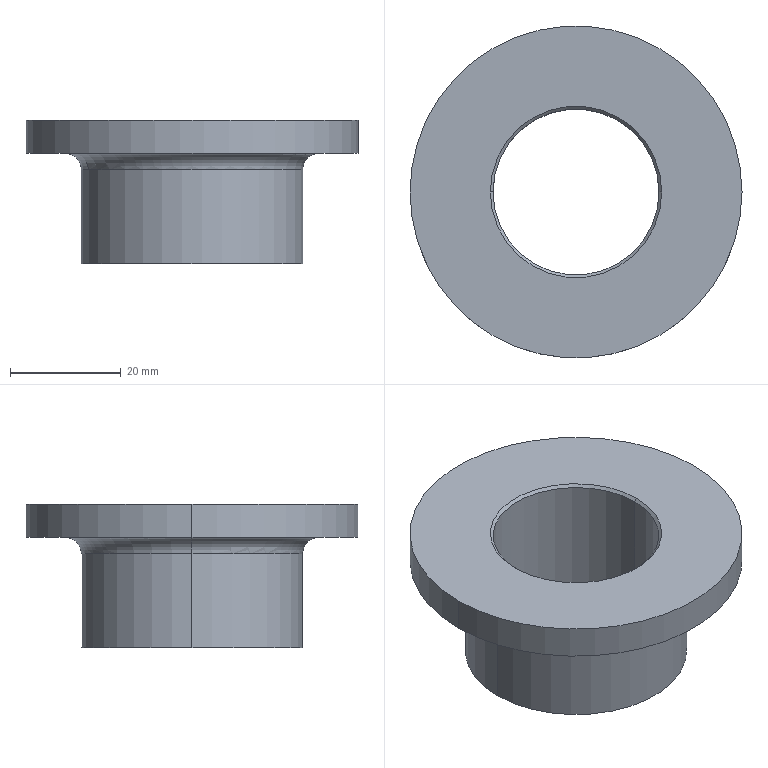Part | SolidWorks | features Chamfer 1, Extrusion 1, Fillet 1, ICE 1 | 1 solid | 15 faces | box 60 x 60 x 26 mm | volume 23946 mm3 | cylinder 6 | cone 4 | plane 3 | torus 2 | commonest cylinder face diameters 30 x2 40 x2 60 x2
STEP:
#1=CARTESIAN_POINT('',(15.,0.,0.5));
#2=VERTEX_POINT('',#1);
#3=CARTESIAN_POINT('',(-15.,0.,0.5));
#4=VERTEX_POINT('',#3);
#5=CARTESIAN_POINT('',(0.,0.,0.5));
#6=DIRECTION('',(0.,0.,-1.));
#7=DIRECTION('',(1.,0.,0.));
#8=AXIS2_PLACEMENT_3D('',#5,#6,#7);
#9=CIRCLE('',#8,15.);
#10=EDGE_CURVE('',#2,#4,#9,.T.);
#11=ORIENTED_EDGE('',*,*,#10,.F.);
#12=CARTESIAN_POINT('',(15.5,0.,0.));
#13=VERTEX_POINT('',#12);
#14=CARTESIAN_POINT('',(15.5,0.,0.));
#15=DIRECTION('',(0.7071,0.,-0.7071));
#16=VECTOR('',#15,1000.);
#17=LINE('',#14,#16);
#18=EDGE_CURVE('',#2,#13,#17,.T.);
#19=ORIENTED_EDGE('',*,*,#18,.T.);
#20=CARTESIAN_POINT('',(-15.5,0.,0.));
#21=VERTEX_POINT('',#20);
#22=CARTESIAN_POINT('',(0.,0.,0.));
#23=DIRECTION('',(0.,0.,1.));
#24=DIRECTION('',(1.,0.,0.));
#25=AXIS2_PLACEMENT_3D('',#22,#23,#24);
#26=CIRCLE('',#25,15.5);
#27=EDGE_CURVE('',#21,#13,#26,.T.);
#28=ORIENTED_EDGE('',*,*,#27,.F.);
#29=CARTESIAN_POINT('',(-15.5,0.,0.));
#30=DIRECTION('',(-0.7071,0.,-0.7071));
#31=VECTOR('',#30,1000.);
#32=LINE('',#29,#31);
#33=EDGE_CURVE('',#4,#21,#32,.T.);
#34=ORIENTED_EDGE('',*,*,#33,.F.);
#35=EDGE_LOOP('',(#11,#19,#28,#34));
#36=FACE_OUTER_BOUND('',#35,.T.);
#37=CARTESIAN_POINT('',(0.,0.,0.));
#38=DIRECTION('',(0.,0.,-1.));
#39=DIRECTION('',(-1.,0.,0.));
#40=AXIS2_PLACEMENT_3D('',#37,#38,#39);
#41=CONICAL_SURFACE('',#40,15.5,0.7854);
#42=ADVANCED_FACE('',(#36),#41,.F.);
#43=CARTESIAN_POINT('',(-15.,0.,25.5));
#44=VERTEX_POINT('',#43);
#45=CARTESIAN_POINT('',(15.,0.,25.5));
#46=VERTEX_POINT('',#45);
#47=CARTESIAN_POINT('',(0.,0.,25.5));
#48=DIRECTION('',(0.,0.,1.));
#49=DIRECTION('',(1.,0.,0.));
#50=AXIS2_PLACEMENT_3D('',#47,#48,#49);
#51=CIRCLE('',#50,15.);
#52=EDGE_CURVE('',#44,#46,#51,.T.);
#53=ORIENTED_EDGE('',*,*,#52,.F.);
#54=CARTESIAN_POINT('',(-15.5,0.,26.));
#55=VERTEX_POINT('',#54);
#56=CARTESIAN_POINT('',(-15.,0.,25.5));
#57=DIRECTION('',(-0.7071,0.,0.7071));
#58=VECTOR('',#57,1000.);
#59=LINE('',#56,#58);
#60=EDGE_CURVE('',#44,#55,#59,.T.);
#61=ORIENTED_EDGE('',*,*,#60,.T.);
#62=CARTESIAN_POINT('',(15.5,0.,26.));
#63=VERTEX_POINT('',#62);
#64=CARTESIAN_POINT('',(0.,0.,26.));
#65=DIRECTION('',(0.,0.,-1.));
#66=DIRECTION('',(1.,0.,0.));
#67=AXIS2_PLACEMENT_3D('',#64,#65,#66);
#68=CIRCLE('',#67,15.5);
#69=EDGE_CURVE('',#63,#55,#68,.T.);
#70=ORIENTED_EDGE('',*,*,#69,.F.);
#71=CARTESIAN_POINT('',(15.,0.,25.5));
#72=DIRECTION('',(0.7071,0.,0.7071));
#73=VECTOR('',#72,1000.);
#74=LINE('',#71,#73);
#75=EDGE_CURVE('',#46,#63,#74,.T.);
#76=ORIENTED_EDGE('',*,*,#75,.F.);
#77=EDGE_LOOP('',(#53,#61,#70,#76));
#78=FACE_OUTER_BOUND('',#77,.T.);
#79=CARTESIAN_POINT('',(0.,0.,25.5));
#80=DIRECTION('',(0.,0.,1.));
#81=DIRECTION('',(1.,0.,0.));
#82=AXIS2_PLACEMENT_3D('',#79,#80,#81);
#83=CONICAL_SURFACE('',#82,15.,0.7854);
#84=ADVANCED_FACE('',(#78),#83,.F.);
#85=CARTESIAN_POINT('',(-23.,0.,20.));
#86=VERTEX_POINT('',#85);
#87=CARTESIAN_POINT('',(23.,0.,20.));
#88=VERTEX_POINT('',#87);
#89=CARTESIAN_POINT('',(0.,0.,20.));
#90=DIRECTION('',(0.,0.,1.));
#91=DIRECTION('',(1.,0.,0.));
#92=AXIS2_PLACEMENT_3D('',#89,#90,#91);
#93=CIRCLE('',#92,23.);
#94=EDGE_CURVE('',#86,#88,#93,.T.);
#95=ORIENTED_EDGE('',*,*,#94,.F.);
#96=CARTESIAN_POINT('',(-20.,0.,17.));
#97=VERTEX_POINT('',#96);
#98=CARTESIAN_POINT('',(-23.,0.,17.));
#99=DIRECTION('',(0.,1.,0.));
#100=DIRECTION('',(-1.,0.,0.));
#101=AXIS2_PLACEMENT_3D('',#98,#99,#100);
#102=CIRCLE('',#101,3.);
#103=EDGE_CURVE('',#86,#97,#102,.T.);
#104=ORIENTED_EDGE('',*,*,#103,.T.);
#105=CARTESIAN_POINT('',(20.,0.,17.));
#106=VERTEX_POINT('',#105);
#107=CARTESIAN_POINT('',(0.,0.,17.));
#108=DIRECTION('',(0.,0.,-1.));
#109=DIRECTION('',(1.,0.,0.));
#110=AXIS2_PLACEMENT_3D('',#107,#108,#109);
#111=CIRCLE('',#110,20.);
#112=EDGE_CURVE('',#106,#97,#111,.T.);
#113=ORIENTED_EDGE('',*,*,#112,.F.);
#114=CARTESIAN_POINT('',(23.,0.,17.));
#115=DIRECTION('',(0.,-1.,0.));
#116=DIRECTION('',(0.,0.,-1.));
#117=AXIS2_PLACEMENT_3D('',#114,#115,#116);
#118=CIRCLE('',#117,3.);
#119=EDGE_CURVE('',#88,#106,#118,.T.);
#120=ORIENTED_EDGE('',*,*,#119,.F.);
#121=EDGE_LOOP('',(#95,#104,#113,#120));
#122=FACE_OUTER_BOUND('',#121,.T.);
#123=CARTESIAN_POINT('',(0.,0.,17.));
#124=DIRECTION('',(0.,0.,1.));
#125=DIRECTION('',(1.,0.,0.));
#126=AXIS2_PLACEMENT_3D('',#123,#124,#125);
#127=TOROIDAL_SURFACE('',#126,23.,3.);
#128=ADVANCED_FACE('',(#122),#127,.F.);
#129=CARTESIAN_POINT('',(30.,0.,20.));
#130=VERTEX_POINT('',#129);
#131=CARTESIAN_POINT('',(-30.,0.,20.));
#132=VERTEX_POINT('',#131);
#133=CARTESIAN_POINT('',(0.,0.,20.));
#134=DIRECTION('',(0.,0.,1.));
#135=DIRECTION('',(1.,0.,0.));
#136=AXIS2_PLACEMENT_3D('',#133,#134,#135);
#137=CIRCLE('',#136,30.);
#138=EDGE_CURVE('',#130,#132,#137,.T.);
#139=ORIENTED_EDGE('',*,*,#138,.T.);
#140=CARTESIAN_POINT('',(-30.,0.,26.));
#141=VERTEX_POINT('',#140);
#142=CARTESIAN_POINT('',(-30.,0.,20.));
#143=DIRECTION('',(0.,0.,1.));
#144=VECTOR('',#143,1000.);
#145=LINE('',#142,#144);
#146=EDGE_CURVE('',#132,#141,#145,.T.);
#147=ORIENTED_EDGE('',*,*,#146,.T.);
#148=CARTESIAN_POINT('',(30.,0.,26.));
#149=VERTEX_POINT('',#148);
#150=CARTESIAN_POINT('',(0.,0.,26.));
#151=DIRECTION('',(0.,0.,1.));
#152=DIRECTION('',(1.,0.,0.));
#153=AXIS2_PLACEMENT_3D('',#150,#151,#152);
#154=CIRCLE('',#153,30.);
#155=EDGE_CURVE('',#149,#141,#154,.T.);
#156=ORIENTED_EDGE('',*,*,#155,.F.);
#157=CARTESIAN_POINT('',(30.,0.,20.));
#158=DIRECTION('',(0.,0.,1.));
#159=VECTOR('',#158,1000.);
#160=LINE('',#157,#159);
#161=EDGE_CURVE('',#130,#149,#160,.T.);
#162=ORIENTED_EDGE('',*,*,#161,.F.);
#163=EDGE_LOOP('',(#139,#147,#156,#162));
#164=FACE_OUTER_BOUND('',#163,.T.);
#165=CARTESIAN_POINT('',(0.,0.,20.));
#166=DIRECTION('',(0.,0.,1.));
#167=DIRECTION('',(1.,0.,0.));
#168=AXIS2_PLACEMENT_3D('',#165,#166,#167);
#169=CYLINDRICAL_SURFACE('',#168,30.);
#170=ADVANCED_FACE('',(#164),#169,.T.);
#171=ORIENTED_EDGE('',*,*,#52,.T.);
#172=CARTESIAN_POINT('',(15.,0.,26.));
#173=DIRECTION('',(0.,0.,-1.));
#174=VECTOR('',#173,1000.);
#175=LINE('',#172,#174);
#176=EDGE_CURVE('',#46,#2,#175,.T.);
#177=ORIENTED_EDGE('',*,*,#176,.T.);
#178=ORIENTED_EDGE('',*,*,#10,.T.);
#179=CARTESIAN_POINT('',(-15.,0.,26.));
#180=DIRECTION('',(0.,0.,-1.));
#181=VECTOR('',#180,1000.);
#182=LINE('',#179,#181);
#183=EDGE_CURVE('',#44,#4,#182,.T.);
#184=ORIENTED_EDGE('',*,*,#183,.F.);
#185=EDGE_LOOP('',(#171,#177,#178,#184));
#186=FACE_OUTER_BOUND('',#185,.T.);
#187=CARTESIAN_POINT('',(0.,0.,26.));
#188=DIRECTION('',(0.,0.,-1.));
#189=DIRECTION('',(-1.,0.,0.));
#190=AXIS2_PLACEMENT_3D('',#187,#188,#189);
#191=CYLINDRICAL_SURFACE('',#190,15.);
#192=ADVANCED_FACE('',(#186),#191,.F.);
#193=CARTESIAN_POINT('',(0.,0.,17.));
#194=DIRECTION('',(0.,0.,-1.));
#195=DIRECTION('',(1.,0.,0.));
#196=AXIS2_PLACEMENT_3D('',#193,#194,#195);
#197=CIRCLE('',#196,20.);
#198=EDGE_CURVE('',#97,#106,#197,.T.);
#199=ORIENTED_EDGE('',*,*,#198,.T.);
#200=CARTESIAN_POINT('',(20.,0.,0.));
#201=VERTEX_POINT('',#200);
#202=CARTESIAN_POINT('',(20.,0.,26.));
#203=DIRECTION('',(0.,0.,-1.));
#204=VECTOR('',#203,1000.);
#205=LINE('',#202,#204);
#206=EDGE_CURVE('',#106,#201,#205,.T.);
#207=ORIENTED_EDGE('',*,*,#206,.T.);
#208=CARTESIAN_POINT('',(-20.,0.,0.));
#209=VERTEX_POINT('',#208);
#210=CARTESIAN_POINT('',(0.,0.,0.));
#211=DIRECTION('',(0.,0.,1.));
#212=DIRECTION('',(1.,0.,0.));
#213=AXIS2_PLACEMENT_3D('',#210,#211,#212);
#214=CIRCLE('',#213,20.);
#215=EDGE_CURVE('',#201,#209,#214,.T.);
#216=ORIENTED_EDGE('',*,*,#215,.T.);
#217=CARTESIAN_POINT('',(-20.,0.,26.));
#218=DIRECTION('',(0.,0.,-1.));
#219=VECTOR('',#218,1000.);
#220=LINE('',#217,#219);
#221=EDGE_CURVE('',#97,#209,#220,.T.);
#222=ORIENTED_EDGE('',*,*,#221,.F.);
#223=EDGE_LOOP('',(#199,#207,#216,#222));
#224=FACE_OUTER_BOUND('',#223,.T.);
#225=CARTESIAN_POINT('',(0.,0.,26.));
#226=DIRECTION('',(0.,0.,-1.));
#227=DIRECTION('',(-1.,0.,0.));
#228=AXIS2_PLACEMENT_3D('',#225,#226,#227);
#229=CYLINDRICAL_SURFACE('',#228,20.);
#230=ADVANCED_FACE('',(#224),#229,.T.);
#231=ORIENTED_EDGE('',*,*,#206,.F.);
#232=ORIENTED_EDGE('',*,*,#112,.T.);
#233=ORIENTED_EDGE('',*,*,#221,.T.);
#234=CARTESIAN_POINT('',(0.,0.,0.));
#235=DIRECTION('',(0.,0.,1.));
#236=DIRECTION('',(1.,0.,0.));
#237=AXIS2_PLACEMENT_3D('',#234,#235,#236);
#238=CIRCLE('',#237,20.);
#239=EDGE_CURVE('',#209,#201,#238,.T.);
#240=ORIENTED_EDGE('',*,*,#239,.T.);
#241=EDGE_LOOP('',(#231,#232,#233,#240));
#242=FACE_OUTER_BOUND('',#241,.T.);
#243=CARTESIAN_POINT('',(0.,0.,26.));
#244=DIRECTION('',(0.,0.,-1.));
#245=DIRECTION('',(-1.,0.,0.));
#246=AXIS2_PLACEMENT_3D('',#243,#244,#245);
#247=CYLINDRICAL_SURFACE('',#246,20.);
#248=ADVANCED_FACE('',(#242),#247,.T.);
#249=ORIENTED_EDGE('',*,*,#69,.T.);
#250=CARTESIAN_POINT('',(0.,0.,26.));
#251=DIRECTION('',(0.,0.,-1.));
#252=DIRECTION('',(1.,0.,0.));
#253=AXIS2_PLACEMENT_3D('',#250,#251,#252);
#254=CIRCLE('',#253,15.5);
#255=EDGE_CURVE('',#55,#63,#254,.T.);
#256=ORIENTED_EDGE('',*,*,#255,.T.);
#257=EDGE_LOOP('',(#249,#256));
#258=FACE_BOUND('',#257,.T.);
#259=ORIENTED_EDGE('',*,*,#155,.T.);
#260=CARTESIAN_POINT('',(0.,0.,26.));
#261=DIRECTION('',(0.,0.,1.));
#262=DIRECTION('',(1.,0.,0.));
#263=AXIS2_PLACEMENT_3D('',#260,#261,#262);
#264=CIRCLE('',#263,30.);
#265=EDGE_CURVE('',#141,#149,#264,.T.);
#266=ORIENTED_EDGE('',*,*,#265,.T.);
#267=EDGE_LOOP('',(#259,#266));
#268=FACE_OUTER_BOUND('',#267,.T.);
#269=CARTESIAN_POINT('',(0.,0.,26.));
#270=DIRECTION('',(0.,0.,1.));
#271=DIRECTION('',(1.,0.,0.));
#272=AXIS2_PLACEMENT_3D('',#269,#270,#271);
#273=PLANE('',#272);
#274=ADVANCED_FACE('',(#258,#268),#273,.T.);
#275=ORIENTED_EDGE('',*,*,#27,.T.);
#276=CARTESIAN_POINT('',(0.,0.,0.));
#277=DIRECTION('',(0.,0.,1.));
#278=DIRECTION('',(1.,0.,0.));
#279=AXIS2_PLACEMENT_3D('',#276,#277,#278);
#280=CIRCLE('',#279,15.5);
#281=EDGE_CURVE('',#13,#21,#280,.T.);
#282=ORIENTED_EDGE('',*,*,#281,.T.);
#283=EDGE_LOOP('',(#275,#282));
#284=FACE_BOUND('',#283,.T.);
#285=ORIENTED_EDGE('',*,*,#239,.F.);
#286=ORIENTED_EDGE('',*,*,#215,.F.);
#287=EDGE_LOOP('',(#285,#286));
#288=FACE_OUTER_BOUND('',#287,.T.);
#289=CARTESIAN_POINT('',(0.,0.,0.));
#290=DIRECTION('',(0.,0.,1.));
#291=DIRECTION('',(1.,0.,0.));
#292=AXIS2_PLACEMENT_3D('',#289,#290,#291);
#293=PLANE('',#292);
#294=ADVANCED_FACE('',(#284,#288),#293,.F.);
#295=ORIENTED_EDGE('',*,*,#176,.F.);
#296=CARTESIAN_POINT('',(0.,0.,25.5));
#297=DIRECTION('',(0.,0.,1.));
#298=DIRECTION('',(1.,0.,0.));
#299=AXIS2_PLACEMENT_3D('',#296,#297,#298);
#300=CIRCLE('',#299,15.);
#301=EDGE_CURVE('',#46,#44,#300,.T.);
#302=ORIENTED_EDGE('',*,*,#301,.T.);
#303=ORIENTED_EDGE('',*,*,#183,.T.);
#304=CARTESIAN_POINT('',(0.,0.,0.5));
#305=DIRECTION('',(0.,0.,-1.));
#306=DIRECTION('',(1.,0.,0.));
#307=AXIS2_PLACEMENT_3D('',#304,#305,#306);
#308=CIRCLE('',#307,15.);
#309=EDGE_CURVE('',#4,#2,#308,.T.);
#310=ORIENTED_EDGE('',*,*,#309,.T.);
#311=EDGE_LOOP('',(#295,#302,#303,#310));
#312=FACE_OUTER_BOUND('',#311,.T.);
#313=CARTESIAN_POINT('',(0.,0.,26.));
#314=DIRECTION('',(0.,0.,-1.));
#315=DIRECTION('',(-1.,0.,0.));
#316=AXIS2_PLACEMENT_3D('',#313,#314,#315);
#317=CYLINDRICAL_SURFACE('',#316,15.);
#318=ADVANCED_FACE('',(#312),#317,.F.);
#319=CARTESIAN_POINT('',(0.,0.,20.));
#320=DIRECTION('',(0.,0.,1.));
#321=DIRECTION('',(1.,0.,0.));
#322=AXIS2_PLACEMENT_3D('',#319,#320,#321);
#323=CIRCLE('',#322,23.);
#324=EDGE_CURVE('',#88,#86,#323,.T.);
#325=ORIENTED_EDGE('',*,*,#324,.T.);
#326=ORIENTED_EDGE('',*,*,#94,.T.);
#327=EDGE_LOOP('',(#325,#326));
#328=FACE_BOUND('',#327,.T.);
#329=ORIENTED_EDGE('',*,*,#138,.F.);
#330=CARTESIAN_POINT('',(0.,0.,20.));
#331=DIRECTION('',(0.,0.,1.));
#332=DIRECTION('',(1.,0.,0.));
#333=AXIS2_PLACEMENT_3D('',#330,#331,#332);
#334=CIRCLE('',#333,30.);
#335=EDGE_CURVE('',#132,#130,#334,.T.);
#336=ORIENTED_EDGE('',*,*,#335,.F.);
#337=EDGE_LOOP('',(#329,#336));
#338=FACE_OUTER_BOUND('',#337,.T.);
#339=CARTESIAN_POINT('',(0.,0.,20.));
#340=DIRECTION('',(0.,0.,1.));
#341=DIRECTION('',(1.,0.,0.));
#342=AXIS2_PLACEMENT_3D('',#339,#340,#341);
#343=PLANE('',#342);
#344=ADVANCED_FACE('',(#328,#338),#343,.F.);
#345=ORIENTED_EDGE('',*,*,#146,.F.);
#346=ORIENTED_EDGE('',*,*,#335,.T.);
#347=ORIENTED_EDGE('',*,*,#161,.T.);
#348=ORIENTED_EDGE('',*,*,#265,.F.);
#349=EDGE_LOOP('',(#345,#346,#347,#348));
#350=FACE_OUTER_BOUND('',#349,.T.);
#351=CARTESIAN_POINT('',(0.,0.,20.));
#352=DIRECTION('',(0.,0.,1.));
#353=DIRECTION('',(1.,0.,0.));
#354=AXIS2_PLACEMENT_3D('',#351,#352,#353);
#355=CYLINDRICAL_SURFACE('',#354,30.);
#356=ADVANCED_FACE('',(#350),#355,.T.);
#357=ORIENTED_EDGE('',*,*,#103,.F.);
#358=ORIENTED_EDGE('',*,*,#324,.F.);
#359=ORIENTED_EDGE('',*,*,#119,.T.);
#360=ORIENTED_EDGE('',*,*,#198,.F.);
#361=EDGE_LOOP('',(#357,#358,#359,#360));
#362=FACE_OUTER_BOUND('',#361,.T.);
#363=CARTESIAN_POINT('',(0.,0.,17.));
#364=DIRECTION('',(0.,0.,1.));
#365=DIRECTION('',(1.,0.,0.));
#366=AXIS2_PLACEMENT_3D('',#363,#364,#365);
#367=TOROIDAL_SURFACE('',#366,23.,3.);
#368=ADVANCED_FACE('',(#362),#367,.F.);
#369=ORIENTED_EDGE('',*,*,#60,.F.);
#370=ORIENTED_EDGE('',*,*,#301,.F.);
#371=ORIENTED_EDGE('',*,*,#75,.T.);
#372=ORIENTED_EDGE('',*,*,#255,.F.);
#373=EDGE_LOOP('',(#369,#370,#371,#372));
#374=FACE_OUTER_BOUND('',#373,.T.);
#375=CARTESIAN_POINT('',(0.,0.,25.5));
#376=DIRECTION('',(0.,0.,1.));
#377=DIRECTION('',(1.,0.,0.));
#378=AXIS2_PLACEMENT_3D('',#375,#376,#377);
#379=CONICAL_SURFACE('',#378,15.,0.7854);
#380=ADVANCED_FACE('',(#374),#379,.F.);
#381=ORIENTED_EDGE('',*,*,#18,.F.);
#382=ORIENTED_EDGE('',*,*,#309,.F.);
#383=ORIENTED_EDGE('',*,*,#33,.T.);
#384=ORIENTED_EDGE('',*,*,#281,.F.);
#385=EDGE_LOOP('',(#381,#382,#383,#384));
#386=FACE_OUTER_BOUND('',#385,.T.);
#387=CARTESIAN_POINT('',(0.,0.,0.));
#388=DIRECTION('',(0.,0.,-1.));
#389=DIRECTION('',(-1.,0.,0.));
#390=AXIS2_PLACEMENT_3D('',#387,#388,#389);
#391=CONICAL_SURFACE('',#390,15.5,0.7854);
#392=ADVANCED_FACE('',(#386),#391,.F.);
#393=CLOSED_SHELL('',(#42,#84,#128,#170,#192,#230,#248,#274,#294,#318,#344,#356,#368,#380,#392));
#394=MANIFOLD_SOLID_BREP('',#393);
#395=CARTESIAN_POINT('',(0.,0.,0.));
#396=DIRECTION('',(0.,0.,1.));
#397=DIRECTION('',(1.,0.,0.));
#398=AXIS2_PLACEMENT_3D('',#395,#396,#397);
#399=(LENGTH_UNIT()NAMED_UNIT(*)SI_UNIT(.MILLI.,.METRE.));
#400=UNCERTAINTY_MEASURE_WITH_UNIT(LENGTH_MEASURE(0.00001),#399,'','');
#401=(NAMED_UNIT(*)PLANE_ANGLE_UNIT()SI_UNIT($,.RADIAN.));
#402=(NAMED_UNIT(*)SI_UNIT($,.STERADIAN.)SOLID_ANGLE_UNIT());
#403=(GEOMETRIC_REPRESENTATION_CONTEXT(3)GLOBAL_UNCERTAINTY_ASSIGNED_CONTEXT((#400))GLOBAL_UNIT_ASSIGNED_CONTEXT((#399,#401,#402))REPRESENTATION_CONTEXT('',''));
#404=ADVANCED_BREP_SHAPE_REPRESENTATION('',(#394,#398),#403);